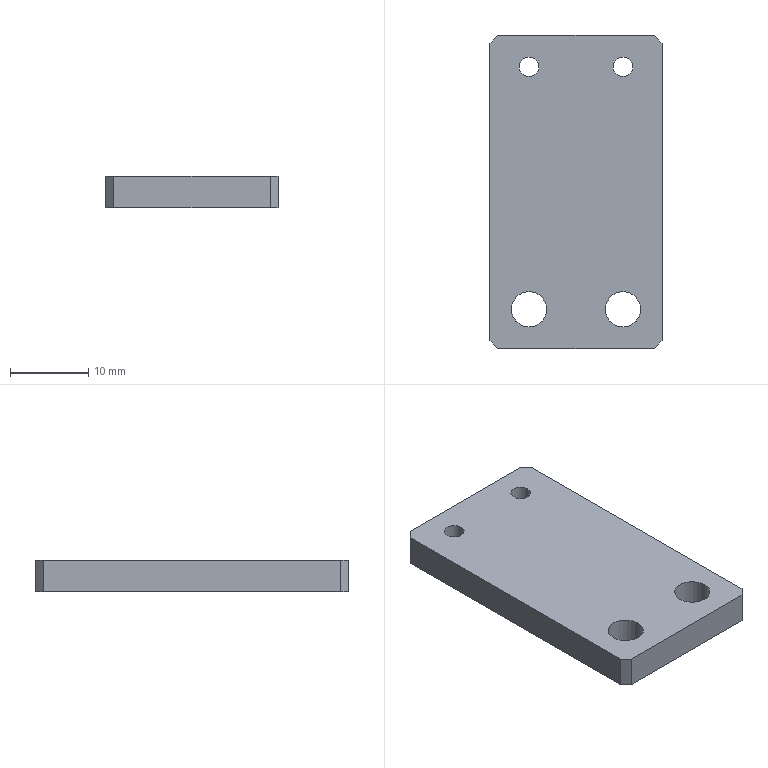Part | NX | 1 solid | 14 faces | box 22 x 40 x 4 mm | volume 3345 mm3 | plane 10 | cylinder 4 | commonest cylinder face diameters 2.5 x2 4.5 x2
STEP:
#1=CARTESIAN_POINT('',(-4.75,16.,0.));
#2=VERTEX_POINT('',#1);
#3=CARTESIAN_POINT('',(-6.,16.,0.));
#4=DIRECTION('',(0.,0.,1.));
#5=DIRECTION('',(1.,0.,0.));
#6=AXIS2_PLACEMENT_3D('',#3,#4,#5);
#7=CIRCLE('',#6,1.25);
#8=EDGE_CURVE('',#2,#2,#7,.T.);
#9=ORIENTED_EDGE('',*,*,#8,.F.);
#10=EDGE_LOOP('',(#9));
#11=FACE_BOUND('',#10,.T.);
#12=CARTESIAN_POINT('',(7.25,16.,0.));
#13=VERTEX_POINT('',#12);
#14=CARTESIAN_POINT('',(6.,16.,0.));
#15=DIRECTION('',(0.,0.,1.));
#16=DIRECTION('',(1.,0.,0.));
#17=AXIS2_PLACEMENT_3D('',#14,#15,#16);
#18=CIRCLE('',#17,1.25);
#19=EDGE_CURVE('',#13,#13,#18,.T.);
#20=ORIENTED_EDGE('',*,*,#19,.F.);
#21=EDGE_LOOP('',(#20));
#22=FACE_BOUND('',#21,.T.);
#23=CARTESIAN_POINT('',(-10.,-20.,0.));
#24=VERTEX_POINT('',#23);
#25=CARTESIAN_POINT('',(10.,-20.,0.));
#26=VERTEX_POINT('',#25);
#27=CARTESIAN_POINT('',(-11.,-20.,0.));
#28=DIRECTION('',(1.,0.,0.));
#29=VECTOR('',#28,1000.);
#30=LINE('',#27,#29);
#31=EDGE_CURVE('',#24,#26,#30,.T.);
#32=ORIENTED_EDGE('',*,*,#31,.T.);
#33=CARTESIAN_POINT('',(11.,-19.,0.));
#34=VERTEX_POINT('',#33);
#35=CARTESIAN_POINT('',(10.,-20.,0.));
#36=DIRECTION('',(-0.7071,-0.7071,0.));
#37=VECTOR('',#36,1000.);
#38=LINE('',#35,#37);
#39=EDGE_CURVE('',#26,#34,#38,.F.);
#40=ORIENTED_EDGE('',*,*,#39,.T.);
#41=CARTESIAN_POINT('',(11.,19.,0.));
#42=VERTEX_POINT('',#41);
#43=CARTESIAN_POINT('',(11.,-20.,0.));
#44=DIRECTION('',(0.,1.,0.));
#45=VECTOR('',#44,1000.);
#46=LINE('',#43,#45);
#47=EDGE_CURVE('',#34,#42,#46,.T.);
#48=ORIENTED_EDGE('',*,*,#47,.T.);
#49=CARTESIAN_POINT('',(10.,20.,0.));
#50=VERTEX_POINT('',#49);
#51=CARTESIAN_POINT('',(11.,19.,0.));
#52=DIRECTION('',(0.7071,-0.7071,0.));
#53=VECTOR('',#52,1000.);
#54=LINE('',#51,#53);
#55=EDGE_CURVE('',#42,#50,#54,.F.);
#56=ORIENTED_EDGE('',*,*,#55,.T.);
#57=CARTESIAN_POINT('',(-10.,20.,0.));
#58=VERTEX_POINT('',#57);
#59=CARTESIAN_POINT('',(-11.,20.,0.));
#60=DIRECTION('',(-1.,0.,0.));
#61=VECTOR('',#60,1000.);
#62=LINE('',#59,#61);
#63=EDGE_CURVE('',#50,#58,#62,.T.);
#64=ORIENTED_EDGE('',*,*,#63,.T.);
#65=CARTESIAN_POINT('',(-11.,19.,0.));
#66=VERTEX_POINT('',#65);
#67=CARTESIAN_POINT('',(-10.,20.,0.));
#68=DIRECTION('',(0.7071,0.7071,0.));
#69=VECTOR('',#68,1000.);
#70=LINE('',#67,#69);
#71=EDGE_CURVE('',#58,#66,#70,.F.);
#72=ORIENTED_EDGE('',*,*,#71,.T.);
#73=CARTESIAN_POINT('',(-11.,-19.,0.));
#74=VERTEX_POINT('',#73);
#75=CARTESIAN_POINT('',(-11.,-20.,0.));
#76=DIRECTION('',(0.,-1.,0.));
#77=VECTOR('',#76,1000.);
#78=LINE('',#75,#77);
#79=EDGE_CURVE('',#66,#74,#78,.T.);
#80=ORIENTED_EDGE('',*,*,#79,.T.);
#81=CARTESIAN_POINT('',(-11.,-19.,0.));
#82=DIRECTION('',(-0.7071,0.7071,0.));
#83=VECTOR('',#82,1000.);
#84=LINE('',#81,#83);
#85=EDGE_CURVE('',#74,#24,#84,.F.);
#86=ORIENTED_EDGE('',*,*,#85,.T.);
#87=EDGE_LOOP('',(#32,#40,#48,#56,#64,#72,#80,#86));
#88=FACE_BOUND('',#87,.T.);
#89=CARTESIAN_POINT('',(8.25,-15.,0.));
#90=VERTEX_POINT('',#89);
#91=CARTESIAN_POINT('',(6.,-15.,0.));
#92=DIRECTION('',(0.,0.,1.));
#93=DIRECTION('',(1.,0.,0.));
#94=AXIS2_PLACEMENT_3D('',#91,#92,#93);
#95=CIRCLE('',#94,2.25);
#96=EDGE_CURVE('',#90,#90,#95,.T.);
#97=ORIENTED_EDGE('',*,*,#96,.F.);
#98=EDGE_LOOP('',(#97));
#99=FACE_BOUND('',#98,.T.);
#100=CARTESIAN_POINT('',(-3.75,-15.,0.));
#101=VERTEX_POINT('',#100);
#102=CARTESIAN_POINT('',(-6.,-15.,0.));
#103=DIRECTION('',(0.,0.,1.));
#104=DIRECTION('',(1.,0.,0.));
#105=AXIS2_PLACEMENT_3D('',#102,#103,#104);
#106=CIRCLE('',#105,2.25);
#107=EDGE_CURVE('',#101,#101,#106,.T.);
#108=ORIENTED_EDGE('',*,*,#107,.F.);
#109=EDGE_LOOP('',(#108));
#110=FACE_BOUND('',#109,.T.);
#111=CARTESIAN_POINT('',(0.,0.,0.));
#112=DIRECTION('',(0.,0.,-1.));
#113=DIRECTION('',(-1.,0.,0.));
#114=AXIS2_PLACEMENT_3D('',#111,#112,#113);
#115=PLANE('',#114);
#116=ADVANCED_FACE('',(#11,#22,#88,#99,#110),#115,.F.);
#117=ORIENTED_EDGE('',*,*,#47,.F.);
#118=CARTESIAN_POINT('',(11.,-19.,-4.));
#119=VERTEX_POINT('',#118);
#120=CARTESIAN_POINT('',(11.,-19.,-4.));
#121=DIRECTION('',(0.,0.,-1.));
#122=VECTOR('',#121,1000.);
#123=LINE('',#120,#122);
#124=EDGE_CURVE('',#34,#119,#123,.T.);
#125=ORIENTED_EDGE('',*,*,#124,.T.);
#126=CARTESIAN_POINT('',(11.,19.,-4.));
#127=VERTEX_POINT('',#126);
#128=CARTESIAN_POINT('',(11.,-20.,-4.));
#129=DIRECTION('',(0.,1.,0.));
#130=VECTOR('',#129,1000.);
#131=LINE('',#128,#130);
#132=EDGE_CURVE('',#119,#127,#131,.T.);
#133=ORIENTED_EDGE('',*,*,#132,.T.);
#134=CARTESIAN_POINT('',(11.,19.,-4.));
#135=DIRECTION('',(0.,0.,1.));
#136=VECTOR('',#135,1000.);
#137=LINE('',#134,#136);
#138=EDGE_CURVE('',#127,#42,#137,.T.);
#139=ORIENTED_EDGE('',*,*,#138,.T.);
#140=EDGE_LOOP('',(#117,#125,#133,#139));
#141=FACE_BOUND('',#140,.T.);
#142=CARTESIAN_POINT('',(11.,-20.,-4.));
#143=DIRECTION('',(1.,0.,0.));
#144=DIRECTION('',(0.,0.,-1.));
#145=AXIS2_PLACEMENT_3D('',#142,#143,#144);
#146=PLANE('',#145);
#147=ADVANCED_FACE('',(#141),#146,.T.);
#148=CARTESIAN_POINT('',(-10.,-20.,-4.));
#149=VERTEX_POINT('',#148);
#150=CARTESIAN_POINT('',(10.,-20.,-4.));
#151=VERTEX_POINT('',#150);
#152=CARTESIAN_POINT('',(-11.,-20.,-4.));
#153=DIRECTION('',(1.,0.,0.));
#154=VECTOR('',#153,1000.);
#155=LINE('',#152,#154);
#156=EDGE_CURVE('',#149,#151,#155,.T.);
#157=ORIENTED_EDGE('',*,*,#156,.T.);
#158=CARTESIAN_POINT('',(10.,-20.,-4.));
#159=DIRECTION('',(0.,0.,1.));
#160=VECTOR('',#159,1000.);
#161=LINE('',#158,#160);
#162=EDGE_CURVE('',#151,#26,#161,.T.);
#163=ORIENTED_EDGE('',*,*,#162,.T.);
#164=ORIENTED_EDGE('',*,*,#31,.F.);
#165=CARTESIAN_POINT('',(-10.,-20.,-4.));
#166=DIRECTION('',(0.,0.,-1.));
#167=VECTOR('',#166,1000.);
#168=LINE('',#165,#167);
#169=EDGE_CURVE('',#24,#149,#168,.T.);
#170=ORIENTED_EDGE('',*,*,#169,.T.);
#171=EDGE_LOOP('',(#157,#163,#164,#170));
#172=FACE_BOUND('',#171,.T.);
#173=CARTESIAN_POINT('',(-11.,-20.,-4.));
#174=DIRECTION('',(0.,-1.,0.));
#175=DIRECTION('',(0.,0.,-1.));
#176=AXIS2_PLACEMENT_3D('',#173,#174,#175);
#177=PLANE('',#176);
#178=ADVANCED_FACE('',(#172),#177,.T.);
#179=CARTESIAN_POINT('',(-11.,19.,-4.));
#180=VERTEX_POINT('',#179);
#181=CARTESIAN_POINT('',(-11.,-19.,-4.));
#182=VERTEX_POINT('',#181);
#183=CARTESIAN_POINT('',(-11.,-20.,-4.));
#184=DIRECTION('',(0.,-1.,0.));
#185=VECTOR('',#184,1000.);
#186=LINE('',#183,#185);
#187=EDGE_CURVE('',#180,#182,#186,.T.);
#188=ORIENTED_EDGE('',*,*,#187,.T.);
#189=CARTESIAN_POINT('',(-11.,-19.,-4.));
#190=DIRECTION('',(0.,0.,1.));
#191=VECTOR('',#190,1000.);
#192=LINE('',#189,#191);
#193=EDGE_CURVE('',#182,#74,#192,.T.);
#194=ORIENTED_EDGE('',*,*,#193,.T.);
#195=ORIENTED_EDGE('',*,*,#79,.F.);
#196=CARTESIAN_POINT('',(-11.,19.,-4.));
#197=DIRECTION('',(0.,0.,-1.));
#198=VECTOR('',#197,1000.);
#199=LINE('',#196,#198);
#200=EDGE_CURVE('',#66,#180,#199,.T.);
#201=ORIENTED_EDGE('',*,*,#200,.T.);
#202=EDGE_LOOP('',(#188,#194,#195,#201));
#203=FACE_BOUND('',#202,.T.);
#204=CARTESIAN_POINT('',(-11.,-20.,-4.));
#205=DIRECTION('',(-1.,0.,0.));
#206=DIRECTION('',(0.,0.,1.));
#207=AXIS2_PLACEMENT_3D('',#204,#205,#206);
#208=PLANE('',#207);
#209=ADVANCED_FACE('',(#203),#208,.T.);
#210=ORIENTED_EDGE('',*,*,#63,.F.);
#211=CARTESIAN_POINT('',(10.,20.,-4.));
#212=VERTEX_POINT('',#211);
#213=CARTESIAN_POINT('',(10.,20.,-4.));
#214=DIRECTION('',(0.,0.,-1.));
#215=VECTOR('',#214,1000.);
#216=LINE('',#213,#215);
#217=EDGE_CURVE('',#50,#212,#216,.T.);
#218=ORIENTED_EDGE('',*,*,#217,.T.);
#219=CARTESIAN_POINT('',(-10.,20.,-4.));
#220=VERTEX_POINT('',#219);
#221=CARTESIAN_POINT('',(-11.,20.,-4.));
#222=DIRECTION('',(-1.,0.,0.));
#223=VECTOR('',#222,1000.);
#224=LINE('',#221,#223);
#225=EDGE_CURVE('',#212,#220,#224,.T.);
#226=ORIENTED_EDGE('',*,*,#225,.T.);
#227=CARTESIAN_POINT('',(-10.,20.,-4.));
#228=DIRECTION('',(0.,0.,1.));
#229=VECTOR('',#228,1000.);
#230=LINE('',#227,#229);
#231=EDGE_CURVE('',#220,#58,#230,.T.);
#232=ORIENTED_EDGE('',*,*,#231,.T.);
#233=EDGE_LOOP('',(#210,#218,#226,#232));
#234=FACE_BOUND('',#233,.T.);
#235=CARTESIAN_POINT('',(-11.,20.,-4.));
#236=DIRECTION('',(0.,1.,0.));
#237=DIRECTION('',(0.,0.,1.));
#238=AXIS2_PLACEMENT_3D('',#235,#236,#237);
#239=PLANE('',#238);
#240=ADVANCED_FACE('',(#234),#239,.T.);
#241=CARTESIAN_POINT('',(-4.75,16.,-4.));
#242=VERTEX_POINT('',#241);
#243=CARTESIAN_POINT('',(-6.,16.,-4.));
#244=DIRECTION('',(0.,0.,1.));
#245=DIRECTION('',(1.,0.,0.));
#246=AXIS2_PLACEMENT_3D('',#243,#244,#245);
#247=CIRCLE('',#246,1.25);
#248=EDGE_CURVE('',#242,#242,#247,.T.);
#249=ORIENTED_EDGE('',*,*,#248,.T.);
#250=EDGE_LOOP('',(#249));
#251=FACE_BOUND('',#250,.T.);
#252=CARTESIAN_POINT('',(7.25,16.,-4.));
#253=VERTEX_POINT('',#252);
#254=CARTESIAN_POINT('',(6.,16.,-4.));
#255=DIRECTION('',(0.,0.,1.));
#256=DIRECTION('',(1.,0.,0.));
#257=AXIS2_PLACEMENT_3D('',#254,#255,#256);
#258=CIRCLE('',#257,1.25);
#259=EDGE_CURVE('',#253,#253,#258,.T.);
#260=ORIENTED_EDGE('',*,*,#259,.T.);
#261=EDGE_LOOP('',(#260));
#262=FACE_BOUND('',#261,.T.);
#263=CARTESIAN_POINT('',(-3.75,-15.,-4.));
#264=VERTEX_POINT('',#263);
#265=CARTESIAN_POINT('',(-6.,-15.,-4.));
#266=DIRECTION('',(0.,0.,1.));
#267=DIRECTION('',(1.,0.,0.));
#268=AXIS2_PLACEMENT_3D('',#265,#266,#267);
#269=CIRCLE('',#268,2.25);
#270=EDGE_CURVE('',#264,#264,#269,.T.);
#271=ORIENTED_EDGE('',*,*,#270,.T.);
#272=EDGE_LOOP('',(#271));
#273=FACE_BOUND('',#272,.T.);
#274=CARTESIAN_POINT('',(8.25,-15.,-4.));
#275=VERTEX_POINT('',#274);
#276=CARTESIAN_POINT('',(6.,-15.,-4.));
#277=DIRECTION('',(0.,0.,1.));
#278=DIRECTION('',(1.,0.,0.));
#279=AXIS2_PLACEMENT_3D('',#276,#277,#278);
#280=CIRCLE('',#279,2.25);
#281=EDGE_CURVE('',#275,#275,#280,.T.);
#282=ORIENTED_EDGE('',*,*,#281,.T.);
#283=EDGE_LOOP('',(#282));
#284=FACE_BOUND('',#283,.T.);
#285=ORIENTED_EDGE('',*,*,#132,.F.);
#286=CARTESIAN_POINT('',(15.,-15.,-4.));
#287=DIRECTION('',(0.7071,0.7071,0.));
#288=VECTOR('',#287,1000.);
#289=LINE('',#286,#288);
#290=EDGE_CURVE('',#119,#151,#289,.F.);
#291=ORIENTED_EDGE('',*,*,#290,.T.);
#292=ORIENTED_EDGE('',*,*,#156,.F.);
#293=CARTESIAN_POINT('',(-15.,-15.,-4.));
#294=DIRECTION('',(0.7071,-0.7071,0.));
#295=VECTOR('',#294,1000.);
#296=LINE('',#293,#295);
#297=EDGE_CURVE('',#149,#182,#296,.F.);
#298=ORIENTED_EDGE('',*,*,#297,.T.);
#299=ORIENTED_EDGE('',*,*,#187,.F.);
#300=CARTESIAN_POINT('',(-15.,15.,-4.));
#301=DIRECTION('',(-0.7071,-0.7071,0.));
#302=VECTOR('',#301,1000.);
#303=LINE('',#300,#302);
#304=EDGE_CURVE('',#180,#220,#303,.F.);
#305=ORIENTED_EDGE('',*,*,#304,.T.);
#306=ORIENTED_EDGE('',*,*,#225,.F.);
#307=CARTESIAN_POINT('',(15.,15.,-4.));
#308=DIRECTION('',(-0.7071,0.7071,0.));
#309=VECTOR('',#308,1000.);
#310=LINE('',#307,#309);
#311=EDGE_CURVE('',#212,#127,#310,.F.);
#312=ORIENTED_EDGE('',*,*,#311,.T.);
#313=EDGE_LOOP('',(#285,#291,#292,#298,#299,#305,#306,#312));
#314=FACE_BOUND('',#313,.T.);
#315=CARTESIAN_POINT('',(0.,0.,-4.));
#316=DIRECTION('',(0.,0.,-1.));
#317=DIRECTION('',(-1.,0.,0.));
#318=AXIS2_PLACEMENT_3D('',#315,#316,#317);
#319=PLANE('',#318);
#320=ADVANCED_FACE('',(#251,#262,#273,#284,#314),#319,.T.);
#321=ORIENTED_EDGE('',*,*,#281,.F.);
#322=EDGE_LOOP('',(#321));
#323=FACE_BOUND('',#322,.T.);
#324=ORIENTED_EDGE('',*,*,#96,.T.);
#325=EDGE_LOOP('',(#324));
#326=FACE_BOUND('',#325,.T.);
#327=CARTESIAN_POINT('',(6.,-15.,0.));
#328=DIRECTION('',(0.,0.,1.));
#329=DIRECTION('',(1.,0.,0.));
#330=AXIS2_PLACEMENT_3D('',#327,#328,#329);
#331=CYLINDRICAL_SURFACE('',#330,2.25);
#332=ADVANCED_FACE('',(#323,#326),#331,.F.);
#333=ORIENTED_EDGE('',*,*,#270,.F.);
#334=EDGE_LOOP('',(#333));
#335=FACE_BOUND('',#334,.T.);
#336=ORIENTED_EDGE('',*,*,#107,.T.);
#337=EDGE_LOOP('',(#336));
#338=FACE_BOUND('',#337,.T.);
#339=CARTESIAN_POINT('',(-6.,-15.,0.));
#340=DIRECTION('',(0.,0.,1.));
#341=DIRECTION('',(1.,0.,0.));
#342=AXIS2_PLACEMENT_3D('',#339,#340,#341);
#343=CYLINDRICAL_SURFACE('',#342,2.25);
#344=ADVANCED_FACE('',(#335,#338),#343,.F.);
#345=ORIENTED_EDGE('',*,*,#290,.F.);
#346=ORIENTED_EDGE('',*,*,#124,.F.);
#347=ORIENTED_EDGE('',*,*,#39,.F.);
#348=ORIENTED_EDGE('',*,*,#162,.F.);
#349=EDGE_LOOP('',(#345,#346,#347,#348));
#350=FACE_BOUND('',#349,.T.);
#351=CARTESIAN_POINT('',(10.,-20.,-4.));
#352=DIRECTION('',(-0.7071,0.7071,0.));
#353=DIRECTION('',(0.,0.,1.));
#354=AXIS2_PLACEMENT_3D('',#351,#352,#353);
#355=PLANE('',#354);
#356=ADVANCED_FACE('',(#350),#355,.F.);
#357=ORIENTED_EDGE('',*,*,#297,.F.);
#358=ORIENTED_EDGE('',*,*,#169,.F.);
#359=ORIENTED_EDGE('',*,*,#85,.F.);
#360=ORIENTED_EDGE('',*,*,#193,.F.);
#361=EDGE_LOOP('',(#357,#358,#359,#360));
#362=FACE_BOUND('',#361,.T.);
#363=CARTESIAN_POINT('',(-11.,-19.,-4.));
#364=DIRECTION('',(0.7071,0.7071,0.));
#365=DIRECTION('',(0.,0.,1.));
#366=AXIS2_PLACEMENT_3D('',#363,#364,#365);
#367=PLANE('',#366);
#368=ADVANCED_FACE('',(#362),#367,.F.);
#369=ORIENTED_EDGE('',*,*,#311,.F.);
#370=ORIENTED_EDGE('',*,*,#217,.F.);
#371=ORIENTED_EDGE('',*,*,#55,.F.);
#372=ORIENTED_EDGE('',*,*,#138,.F.);
#373=EDGE_LOOP('',(#369,#370,#371,#372));
#374=FACE_BOUND('',#373,.T.);
#375=CARTESIAN_POINT('',(11.,19.,-4.));
#376=DIRECTION('',(-0.7071,-0.7071,0.));
#377=DIRECTION('',(0.,0.,1.));
#378=AXIS2_PLACEMENT_3D('',#375,#376,#377);
#379=PLANE('',#378);
#380=ADVANCED_FACE('',(#374),#379,.F.);
#381=ORIENTED_EDGE('',*,*,#304,.F.);
#382=ORIENTED_EDGE('',*,*,#200,.F.);
#383=ORIENTED_EDGE('',*,*,#71,.F.);
#384=ORIENTED_EDGE('',*,*,#231,.F.);
#385=EDGE_LOOP('',(#381,#382,#383,#384));
#386=FACE_BOUND('',#385,.T.);
#387=CARTESIAN_POINT('',(-10.,20.,-4.));
#388=DIRECTION('',(0.7071,-0.7071,0.));
#389=DIRECTION('',(0.,0.,1.));
#390=AXIS2_PLACEMENT_3D('',#387,#388,#389);
#391=PLANE('',#390);
#392=ADVANCED_FACE('',(#386),#391,.F.);
#393=ORIENTED_EDGE('',*,*,#259,.F.);
#394=EDGE_LOOP('',(#393));
#395=FACE_BOUND('',#394,.T.);
#396=ORIENTED_EDGE('',*,*,#19,.T.);
#397=EDGE_LOOP('',(#396));
#398=FACE_BOUND('',#397,.T.);
#399=CARTESIAN_POINT('',(6.,16.,0.));
#400=DIRECTION('',(0.,0.,1.));
#401=DIRECTION('',(1.,0.,0.));
#402=AXIS2_PLACEMENT_3D('',#399,#400,#401);
#403=CYLINDRICAL_SURFACE('',#402,1.25);
#404=ADVANCED_FACE('',(#395,#398),#403,.F.);
#405=ORIENTED_EDGE('',*,*,#248,.F.);
#406=EDGE_LOOP('',(#405));
#407=FACE_BOUND('',#406,.T.);
#408=ORIENTED_EDGE('',*,*,#8,.T.);
#409=EDGE_LOOP('',(#408));
#410=FACE_BOUND('',#409,.T.);
#411=CARTESIAN_POINT('',(-6.,16.,0.));
#412=DIRECTION('',(0.,0.,1.));
#413=DIRECTION('',(1.,0.,0.));
#414=AXIS2_PLACEMENT_3D('',#411,#412,#413);
#415=CYLINDRICAL_SURFACE('',#414,1.25);
#416=ADVANCED_FACE('',(#407,#410),#415,.F.);
#417=CLOSED_SHELL('',(#116,#147,#178,#209,#240,#320,#332,#344,#356,#368,#380,#392,#404,#416));
#418=MANIFOLD_SOLID_BREP('',#417);
#419=(LENGTH_UNIT()NAMED_UNIT(*)SI_UNIT(.MILLI.,.METRE.));
#420=UNCERTAINTY_MEASURE_WITH_UNIT(LENGTH_MEASURE(0.00001),#419,'','');
#421=(NAMED_UNIT(*)PLANE_ANGLE_UNIT()SI_UNIT($,.RADIAN.));
#422=(NAMED_UNIT(*)SI_UNIT($,.STERADIAN.)SOLID_ANGLE_UNIT());
#423=(GEOMETRIC_REPRESENTATION_CONTEXT(3)GLOBAL_UNCERTAINTY_ASSIGNED_CONTEXT((#420))GLOBAL_UNIT_ASSIGNED_CONTEXT((#419,#421,#422))REPRESENTATION_CONTEXT('',''));
#424=ADVANCED_BREP_SHAPE_REPRESENTATION('',(#418),#423);